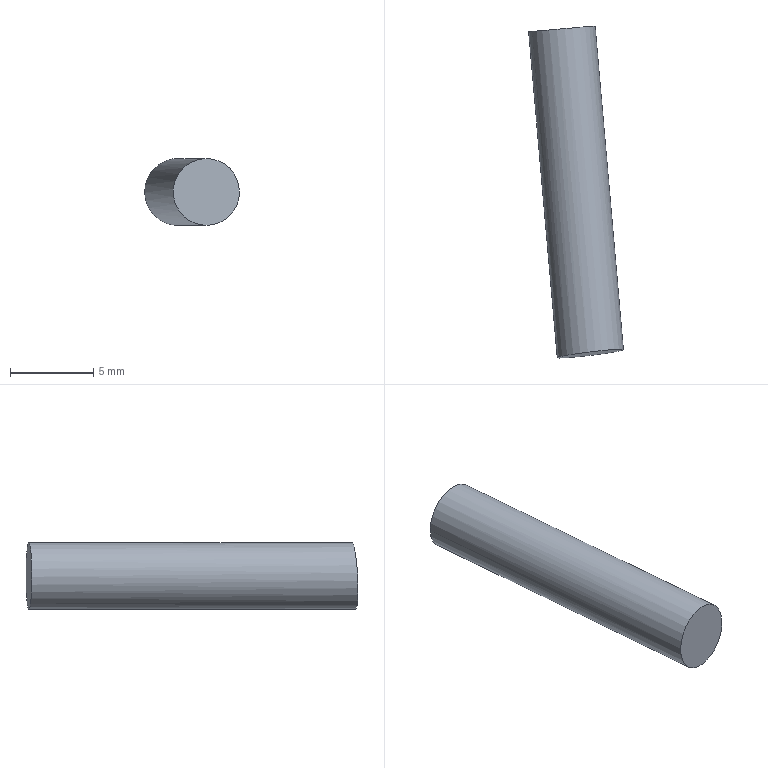Part | NX | features solid 2 | 1 solid | 3 faces | box 5.681 x 19.883 x 4 mm | volume 245.33 mm3 | plane 2 | cylinder 1 | commonest cylinder face diameters 4 x1
STEP:
#1=CARTESIAN_POINT('',(715.403,-34.991,-50.85));
#2=VERTEX_POINT('',#1);
#3=CARTESIAN_POINT('',(713.411,-35.165,-50.85));
#4=DIRECTION('',(0.08716,-0.9962,0.));
#5=DIRECTION('',(0.9962,0.08716,0.));
#6=AXIS2_PLACEMENT_3D('',#3,#4,#5);
#7=CIRCLE('',#6,2.);
#8=EDGE_CURVE('',#2,#2,#7,.T.);
#9=ORIENTED_EDGE('',*,*,#8,.F.);
#10=EDGE_LOOP('',(#9));
#11=FACE_BOUND('',#10,.T.);
#12=CARTESIAN_POINT('',(713.411,-35.165,-50.85));
#13=DIRECTION('',(-0.08716,0.9962,0.));
#14=DIRECTION('',(-0.9962,-0.08716,0.));
#15=AXIS2_PLACEMENT_3D('',#12,#13,#14);
#16=PLANE('',#15);
#17=ADVANCED_FACE('',(#11),#16,.T.);
#18=CARTESIAN_POINT('',(716.177,-54.399,-49.166));
#19=VERTEX_POINT('',#18);
#20=CARTESIAN_POINT('',(715.113,-54.614,-50.85));
#21=DIRECTION('',(-0.1195,0.9915,-0.05097));
#22=DIRECTION('',(0.5313,0.1073,0.8404));
#23=AXIS2_PLACEMENT_3D('',#20,#21,#22);
#24=ELLIPSE('',#23,2.004,2.);
#25=EDGE_CURVE('',#19,#19,#24,.T.);
#26=ORIENTED_EDGE('',*,*,#25,.F.);
#27=EDGE_LOOP('',(#26));
#28=FACE_BOUND('',#27,.T.);
#29=CARTESIAN_POINT('',(707.484,-59.507,-128.15));
#30=DIRECTION('',(-0.1195,0.9915,-0.05097));
#31=DIRECTION('',(0.06611,0.05918,0.9961));
#32=AXIS2_PLACEMENT_3D('',#29,#30,#31);
#33=PLANE('',#32);
#34=ADVANCED_FACE('',(#28),#33,.F.);
#35=ORIENTED_EDGE('',*,*,#8,.T.);
#36=EDGE_LOOP('',(#35));
#37=FACE_BOUND('',#36,.T.);
#38=ORIENTED_EDGE('',*,*,#25,.T.);
#39=EDGE_LOOP('',(#38));
#40=FACE_BOUND('',#39,.T.);
#41=CARTESIAN_POINT('',(715.154,-55.089,-50.85));
#42=DIRECTION('',(-0.08716,0.9962,0.));
#43=DIRECTION('',(-0.9962,-0.08716,0.));
#44=AXIS2_PLACEMENT_3D('',#41,#42,#43);
#45=CYLINDRICAL_SURFACE('',#44,2.);
#46=ADVANCED_FACE('',(#37,#40),#45,.T.);
#47=CLOSED_SHELL('',(#17,#34,#46));
#48=MANIFOLD_SOLID_BREP('',#47);
#49=(LENGTH_UNIT()NAMED_UNIT(*)SI_UNIT(.MILLI.,.METRE.));
#50=UNCERTAINTY_MEASURE_WITH_UNIT(LENGTH_MEASURE(0.00001),#49,'','');
#51=(NAMED_UNIT(*)PLANE_ANGLE_UNIT()SI_UNIT($,.RADIAN.));
#52=(NAMED_UNIT(*)SI_UNIT($,.STERADIAN.)SOLID_ANGLE_UNIT());
#53=(GEOMETRIC_REPRESENTATION_CONTEXT(3)GLOBAL_UNCERTAINTY_ASSIGNED_CONTEXT((#50))GLOBAL_UNIT_ASSIGNED_CONTEXT((#49,#51,#52))REPRESENTATION_CONTEXT('',''));
#54=ADVANCED_BREP_SHAPE_REPRESENTATION('',(#48),#53);